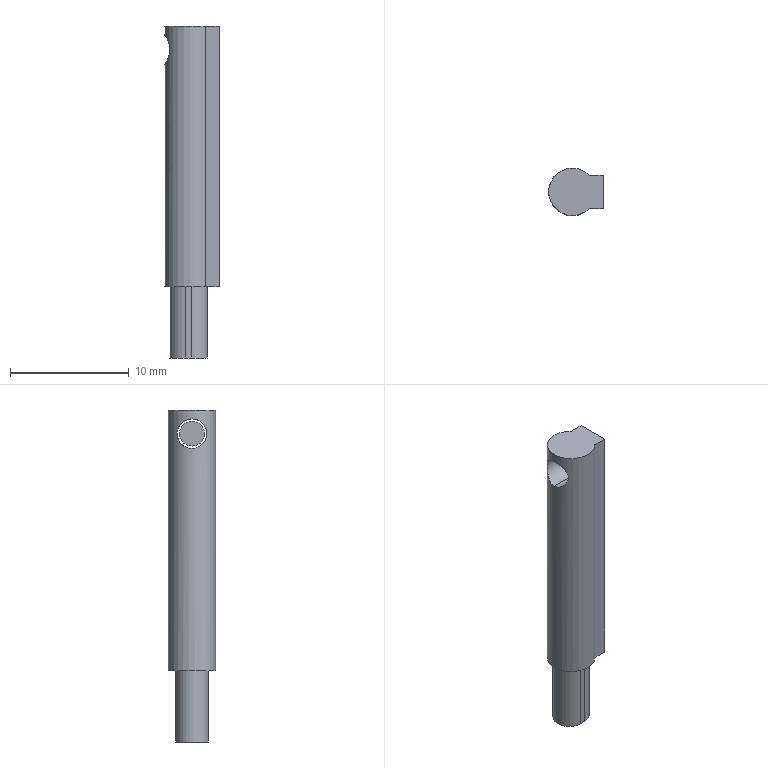Part | SolidWorks | features BaseBody 2 | 2 solids | 18 faces | box 4.6 x 4 x 28 mm | volume 348.237 mm3 | plane 10 | cylinder 8 | commonest cylinder face diameters 2.7 x3 2.1 x2 2.5 x2 4 x1
STEP:
#1=CARTESIAN_POINT('',(14.5,-5.5,-12.25));
#2=VERTEX_POINT('',#1);
#3=CARTESIAN_POINT('',(14.5,-5.5,-14.75));
#4=VERTEX_POINT('',#3);
#5=CARTESIAN_POINT('',(14.5,-5.5,-12.25));
#6=CARTESIAN_POINT('',(14.5,-5.585,-12.25));
#7=CARTESIAN_POINT('',(14.505,-5.668,-12.259));
#8=CARTESIAN_POINT('',(14.526,-5.832,-12.292));
#9=CARTESIAN_POINT('',(14.541,-5.912,-12.317));
#10=CARTESIAN_POINT('',(14.598,-6.138,-12.413));
#11=CARTESIAN_POINT('',(14.651,-6.274,-12.505));
#12=CARTESIAN_POINT('',(14.762,-6.498,-12.73));
#13=CARTESIAN_POINT('',(14.82,-6.588,-12.864));
#14=CARTESIAN_POINT('',(14.909,-6.714,-13.162));
#15=CARTESIAN_POINT('',(14.939,-6.75,-13.33));
#16=CARTESIAN_POINT('',(14.939,-6.75,-13.669));
#17=CARTESIAN_POINT('',(14.91,-6.715,-13.836));
#18=CARTESIAN_POINT('',(14.821,-6.589,-14.135));
#19=CARTESIAN_POINT('',(14.762,-6.498,-14.269));
#20=CARTESIAN_POINT('',(14.651,-6.272,-14.496));
#21=CARTESIAN_POINT('',(14.599,-6.14,-14.586));
#22=CARTESIAN_POINT('',(14.522,-5.835,-14.716));
#23=CARTESIAN_POINT('',(14.5,-5.671,-14.75));
#24=CARTESIAN_POINT('',(14.5,-5.5,-14.75));
#25=B_SPLINE_CURVE_WITH_KNOTS('',3,(#5,#6,#7,#8,#9,#10,#11,#12,#13,#14,#15,#16,#17,#18,#19,#20,#21,#22,#23,#24),.UNSPECIFIED.,.F.,.F.,(4,2,2,2,2,2,2,2,2,4),(0.,0.0002513,0.0005026,0.001005,0.001508,0.00201,0.002513,0.003016,0.003518,0.004021),.UNSPECIFIED.);
#26=EDGE_CURVE('',#2,#4,#25,.T.);
#27=ORIENTED_EDGE('',*,*,#26,.F.);
#28=CARTESIAN_POINT('',(19.1,-5.5,-12.25));
#29=VERTEX_POINT('',#28);
#30=CARTESIAN_POINT('',(19.1,-5.5,-12.25));
#31=DIRECTION('',(1.,0.,0.));
#32=VECTOR('',#31,1000.);
#33=LINE('',#30,#32);
#34=EDGE_CURVE('',#2,#29,#33,.T.);
#35=ORIENTED_EDGE('',*,*,#34,.T.);
#36=CARTESIAN_POINT('',(19.1,-5.5,-14.75));
#37=VERTEX_POINT('',#36);
#38=CARTESIAN_POINT('',(19.1,-5.5,-13.5));
#39=DIRECTION('',(-1.,0.,0.));
#40=DIRECTION('',(0.,0.,-1.));
#41=AXIS2_PLACEMENT_3D('',#38,#39,#40);
#42=CIRCLE('',#41,1.25);
#43=EDGE_CURVE('',#37,#29,#42,.T.);
#44=ORIENTED_EDGE('',*,*,#43,.F.);
#45=CARTESIAN_POINT('',(19.1,-5.5,-14.75));
#46=DIRECTION('',(1.,0.,0.));
#47=VECTOR('',#46,1000.);
#48=LINE('',#45,#47);
#49=EDGE_CURVE('',#4,#37,#48,.T.);
#50=ORIENTED_EDGE('',*,*,#49,.F.);
#51=EDGE_LOOP('',(#27,#35,#44,#50));
#52=FACE_OUTER_BOUND('',#51,.T.);
#53=CARTESIAN_POINT('',(19.1,-5.5,-13.5));
#54=DIRECTION('',(1.,0.,0.));
#55=DIRECTION('',(0.,0.,-1.));
#56=AXIS2_PLACEMENT_3D('',#53,#54,#55);
#57=CYLINDRICAL_SURFACE('',#56,1.25);
#58=ADVANCED_FACE('',(#52),#57,.F.);
#59=CARTESIAN_POINT('',(16.75,-6.85,-39.5));
#60=VERTEX_POINT('',#59);
#61=CARTESIAN_POINT('',(18.1,-5.5,-39.5));
#62=VERTEX_POINT('',#61);
#63=CARTESIAN_POINT('',(16.75,-5.5,-39.5));
#64=DIRECTION('',(0.,0.,1.));
#65=DIRECTION('',(1.,0.,0.));
#66=AXIS2_PLACEMENT_3D('',#63,#64,#65);
#67=CIRCLE('',#66,1.35);
#68=EDGE_CURVE('',#60,#62,#67,.T.);
#69=ORIENTED_EDGE('',*,*,#68,.T.);
#70=CARTESIAN_POINT('',(18.1,-5.5,-33.5));
#71=VERTEX_POINT('',#70);
#72=CARTESIAN_POINT('',(18.1,-5.5,-39.5));
#73=DIRECTION('',(0.,0.,1.));
#74=VECTOR('',#73,1000.);
#75=LINE('',#72,#74);
#76=EDGE_CURVE('',#62,#71,#75,.T.);
#77=ORIENTED_EDGE('',*,*,#76,.T.);
#78=CARTESIAN_POINT('',(16.75,-6.85,-33.5));
#79=VERTEX_POINT('',#78);
#80=CARTESIAN_POINT('',(16.75,-5.5,-33.5));
#81=DIRECTION('',(0.,0.,-1.));
#82=DIRECTION('',(1.,0.,0.));
#83=AXIS2_PLACEMENT_3D('',#80,#81,#82);
#84=CIRCLE('',#83,1.35);
#85=EDGE_CURVE('',#71,#79,#84,.T.);
#86=ORIENTED_EDGE('',*,*,#85,.T.);
#87=CARTESIAN_POINT('',(16.75,-6.85,-39.5));
#88=DIRECTION('',(0.,0.,-1.));
#89=VECTOR('',#88,1000.);
#90=LINE('',#87,#89);
#91=EDGE_CURVE('',#79,#60,#90,.T.);
#92=ORIENTED_EDGE('',*,*,#91,.T.);
#93=EDGE_LOOP('',(#69,#77,#86,#92));
#94=FACE_OUTER_BOUND('',#93,.T.);
#95=CARTESIAN_POINT('',(16.75,-5.5,-39.5));
#96=DIRECTION('',(0.,0.,1.));
#97=DIRECTION('',(1.,0.,0.));
#98=AXIS2_PLACEMENT_3D('',#95,#96,#97);
#99=CYLINDRICAL_SURFACE('',#98,1.35);
#100=ADVANCED_FACE('',(#94),#99,.T.);
#101=CARTESIAN_POINT('',(17.928,-4.1,-33.5));
#102=VERTEX_POINT('',#101);
#103=CARTESIAN_POINT('',(17.928,-6.9,-33.5));
#104=VERTEX_POINT('',#103);
#105=CARTESIAN_POINT('',(16.5,-5.5,-33.5));
#106=DIRECTION('',(0.,0.,1.));
#107=DIRECTION('',(1.,0.,0.));
#108=AXIS2_PLACEMENT_3D('',#105,#106,#107);
#109=CIRCLE('',#108,2.);
#110=EDGE_CURVE('',#102,#104,#109,.T.);
#111=ORIENTED_EDGE('',*,*,#110,.T.);
#112=CARTESIAN_POINT('',(17.928,-6.9,-11.5));
#113=VERTEX_POINT('',#112);
#114=CARTESIAN_POINT('',(17.928,-6.9,-33.5));
#115=DIRECTION('',(0.,0.,1.));
#116=VECTOR('',#115,1000.);
#117=LINE('',#114,#116);
#118=EDGE_CURVE('',#104,#113,#117,.T.);
#119=ORIENTED_EDGE('',*,*,#118,.T.);
#120=CARTESIAN_POINT('',(17.928,-4.1,-11.5));
#121=VERTEX_POINT('',#120);
#122=CARTESIAN_POINT('',(16.5,-5.5,-11.5));
#123=DIRECTION('',(0.,0.,-1.));
#124=DIRECTION('',(1.,0.,0.));
#125=AXIS2_PLACEMENT_3D('',#122,#123,#124);
#126=CIRCLE('',#125,2.);
#127=EDGE_CURVE('',#113,#121,#126,.T.);
#128=ORIENTED_EDGE('',*,*,#127,.T.);
#129=CARTESIAN_POINT('',(17.928,-4.1,-33.5));
#130=DIRECTION('',(0.,0.,-1.));
#131=VECTOR('',#130,1000.);
#132=LINE('',#129,#131);
#133=EDGE_CURVE('',#121,#102,#132,.T.);
#134=ORIENTED_EDGE('',*,*,#133,.T.);
#135=EDGE_LOOP('',(#111,#119,#128,#134));
#136=FACE_OUTER_BOUND('',#135,.T.);
#137=CARTESIAN_POINT('',(14.5,-5.5,-14.75));
#138=CARTESIAN_POINT('',(14.5,-5.415,-14.75));
#139=CARTESIAN_POINT('',(14.505,-5.332,-14.741));
#140=CARTESIAN_POINT('',(14.526,-5.168,-14.708));
#141=CARTESIAN_POINT('',(14.541,-5.088,-14.683));
#142=CARTESIAN_POINT('',(14.598,-4.862,-14.587));
#143=CARTESIAN_POINT('',(14.651,-4.726,-14.495));
#144=CARTESIAN_POINT('',(14.762,-4.502,-14.27));
#145=CARTESIAN_POINT('',(14.82,-4.412,-14.136));
#146=CARTESIAN_POINT('',(14.909,-4.286,-13.838));
#147=CARTESIAN_POINT('',(14.939,-4.25,-13.67));
#148=CARTESIAN_POINT('',(14.939,-4.25,-13.331));
#149=CARTESIAN_POINT('',(14.91,-4.285,-13.164));
#150=CARTESIAN_POINT('',(14.821,-4.411,-12.865));
#151=CARTESIAN_POINT('',(14.762,-4.502,-12.731));
#152=CARTESIAN_POINT('',(14.651,-4.728,-12.504));
#153=CARTESIAN_POINT('',(14.599,-4.86,-12.414));
#154=CARTESIAN_POINT('',(14.541,-5.089,-12.317));
#155=CARTESIAN_POINT('',(14.526,-5.168,-12.292));
#156=CARTESIAN_POINT('',(14.506,-5.33,-12.259));
#157=CARTESIAN_POINT('',(14.5,-5.415,-12.25));
#158=CARTESIAN_POINT('',(14.5,-5.5,-12.25));
#159=B_SPLINE_CURVE_WITH_KNOTS('',3,(#137,#138,#139,#140,#141,#142,#143,#144,#145,#146,#147,#148,#149,#150,#151,#152,#153,#154,#155,#156,#157,#158),.UNSPECIFIED.,.F.,.F.,(4,2,2,2,2,2,2,2,2,2,4),(0.004021,0.004271,0.004522,0.005024,0.005525,0.006027,0.006529,0.00703,0.007532,0.007783,0.008033),.UNSPECIFIED.);
#160=EDGE_CURVE('',#4,#2,#159,.T.);
#161=ORIENTED_EDGE('',*,*,#160,.T.);
#162=ORIENTED_EDGE('',*,*,#26,.T.);
#163=EDGE_LOOP('',(#161,#162));
#164=FACE_BOUND('',#163,.T.);
#165=CARTESIAN_POINT('',(16.5,-5.5,-33.5));
#166=DIRECTION('',(0.,0.,1.));
#167=DIRECTION('',(1.,0.,0.));
#168=AXIS2_PLACEMENT_3D('',#165,#166,#167);
#169=CYLINDRICAL_SURFACE('',#168,2.);
#170=ADVANCED_FACE('',(#136,#164),#169,.T.);
#171=CARTESIAN_POINT('',(19.1,-6.9,-33.5));
#172=VERTEX_POINT('',#171);
#173=CARTESIAN_POINT('',(17.928,-6.9,-33.5));
#174=DIRECTION('',(1.,0.,0.));
#175=VECTOR('',#174,1000.);
#176=LINE('',#173,#175);
#177=EDGE_CURVE('',#104,#172,#176,.T.);
#178=ORIENTED_EDGE('',*,*,#177,.T.);
#179=CARTESIAN_POINT('',(19.1,-6.9,-11.5));
#180=VERTEX_POINT('',#179);
#181=CARTESIAN_POINT('',(19.1,-6.9,-33.5));
#182=DIRECTION('',(0.,0.,1.));
#183=VECTOR('',#182,1000.);
#184=LINE('',#181,#183);
#185=EDGE_CURVE('',#172,#180,#184,.T.);
#186=ORIENTED_EDGE('',*,*,#185,.T.);
#187=CARTESIAN_POINT('',(17.928,-6.9,-11.5));
#188=DIRECTION('',(-1.,0.,0.));
#189=VECTOR('',#188,1000.);
#190=LINE('',#187,#189);
#191=EDGE_CURVE('',#180,#113,#190,.T.);
#192=ORIENTED_EDGE('',*,*,#191,.T.);
#193=ORIENTED_EDGE('',*,*,#118,.F.);
#194=EDGE_LOOP('',(#178,#186,#192,#193));
#195=FACE_OUTER_BOUND('',#194,.T.);
#196=CARTESIAN_POINT('',(17.928,-6.9,-33.5));
#197=DIRECTION('',(0.,-1.,0.));
#198=DIRECTION('',(1.,0.,0.));
#199=AXIS2_PLACEMENT_3D('',#196,#197,#198);
#200=PLANE('',#199);
#201=ADVANCED_FACE('',(#195),#200,.T.);
#202=CARTESIAN_POINT('',(16.25,-6.85,-33.5));
#203=VERTEX_POINT('',#202);
#204=CARTESIAN_POINT('',(16.25,-6.85,-33.5));
#205=DIRECTION('',(1.,0.,0.));
#206=VECTOR('',#205,1000.);
#207=LINE('',#204,#206);
#208=EDGE_CURVE('',#203,#79,#207,.T.);
#209=ORIENTED_EDGE('',*,*,#208,.T.);
#210=ORIENTED_EDGE('',*,*,#85,.F.);
#211=CARTESIAN_POINT('',(16.75,-4.15,-33.5));
#212=VERTEX_POINT('',#211);
#213=CARTESIAN_POINT('',(16.75,-5.5,-33.5));
#214=DIRECTION('',(0.,0.,-1.));
#215=DIRECTION('',(1.,0.,0.));
#216=AXIS2_PLACEMENT_3D('',#213,#214,#215);
#217=CIRCLE('',#216,1.35);
#218=EDGE_CURVE('',#212,#71,#217,.T.);
#219=ORIENTED_EDGE('',*,*,#218,.F.);
#220=CARTESIAN_POINT('',(16.25,-4.15,-33.5));
#221=VERTEX_POINT('',#220);
#222=CARTESIAN_POINT('',(16.75,-4.15,-33.5));
#223=DIRECTION('',(-1.,0.,0.));
#224=VECTOR('',#223,1000.);
#225=LINE('',#222,#224);
#226=EDGE_CURVE('',#212,#221,#225,.T.);
#227=ORIENTED_EDGE('',*,*,#226,.T.);
#228=CARTESIAN_POINT('',(16.25,-5.5,-33.5));
#229=DIRECTION('',(0.,0.,-1.));
#230=DIRECTION('',(1.,0.,0.));
#231=AXIS2_PLACEMENT_3D('',#228,#229,#230);
#232=CIRCLE('',#231,1.35);
#233=EDGE_CURVE('',#203,#221,#232,.T.);
#234=ORIENTED_EDGE('',*,*,#233,.F.);
#235=EDGE_LOOP('',(#209,#210,#219,#227,#234));
#236=FACE_BOUND('',#235,.T.);
#237=ORIENTED_EDGE('',*,*,#110,.F.);
#238=CARTESIAN_POINT('',(19.1,-4.1,-33.5));
#239=VERTEX_POINT('',#238);
#240=CARTESIAN_POINT('',(16.5,-4.1,-33.5));
#241=DIRECTION('',(-1.,0.,0.));
#242=VECTOR('',#241,1000.);
#243=LINE('',#240,#242);
#244=EDGE_CURVE('',#239,#102,#243,.T.);
#245=ORIENTED_EDGE('',*,*,#244,.F.);
#246=CARTESIAN_POINT('',(19.1,-5.5,-33.5));
#247=DIRECTION('',(0.,1.,0.));
#248=VECTOR('',#247,1000.);
#249=LINE('',#246,#248);
#250=EDGE_CURVE('',#172,#239,#249,.T.);
#251=ORIENTED_EDGE('',*,*,#250,.F.);
#252=ORIENTED_EDGE('',*,*,#177,.F.);
#253=EDGE_LOOP('',(#237,#245,#251,#252));
#254=FACE_OUTER_BOUND('',#253,.T.);
#255=CARTESIAN_POINT('',(16.5,-5.5,-33.5));
#256=DIRECTION('',(0.,0.,1.));
#257=DIRECTION('',(1.,0.,0.));
#258=AXIS2_PLACEMENT_3D('',#255,#256,#257);
#259=PLANE('',#258);
#260=ADVANCED_FACE('',(#236,#254),#259,.F.);
#261=ORIENTED_EDGE('',*,*,#244,.T.);
#262=ORIENTED_EDGE('',*,*,#133,.F.);
#263=CARTESIAN_POINT('',(19.1,-4.1,-11.5));
#264=VERTEX_POINT('',#263);
#265=CARTESIAN_POINT('',(19.1,-4.1,-11.5));
#266=DIRECTION('',(1.,0.,0.));
#267=VECTOR('',#266,1000.);
#268=LINE('',#265,#267);
#269=EDGE_CURVE('',#121,#264,#268,.T.);
#270=ORIENTED_EDGE('',*,*,#269,.T.);
#271=CARTESIAN_POINT('',(19.1,-4.1,-33.5));
#272=DIRECTION('',(0.,0.,-1.));
#273=VECTOR('',#272,1000.);
#274=LINE('',#271,#273);
#275=EDGE_CURVE('',#264,#239,#274,.T.);
#276=ORIENTED_EDGE('',*,*,#275,.T.);
#277=EDGE_LOOP('',(#261,#262,#270,#276));
#278=FACE_OUTER_BOUND('',#277,.T.);
#279=CARTESIAN_POINT('',(19.1,-4.1,-33.5));
#280=DIRECTION('',(0.,1.,0.));
#281=DIRECTION('',(-1.,0.,0.));
#282=AXIS2_PLACEMENT_3D('',#279,#280,#281);
#283=PLANE('',#282);
#284=ADVANCED_FACE('',(#278),#283,.T.);
#285=ORIENTED_EDGE('',*,*,#269,.F.);
#286=ORIENTED_EDGE('',*,*,#127,.F.);
#287=ORIENTED_EDGE('',*,*,#191,.F.);
#288=CARTESIAN_POINT('',(19.1,-5.5,-11.5));
#289=DIRECTION('',(0.,1.,0.));
#290=VECTOR('',#289,1000.);
#291=LINE('',#288,#290);
#292=EDGE_CURVE('',#180,#264,#291,.T.);
#293=ORIENTED_EDGE('',*,*,#292,.T.);
#294=EDGE_LOOP('',(#285,#286,#287,#293));
#295=FACE_OUTER_BOUND('',#294,.T.);
#296=CARTESIAN_POINT('',(16.5,-5.5,-11.5));
#297=DIRECTION('',(0.,0.,1.));
#298=DIRECTION('',(1.,0.,0.));
#299=AXIS2_PLACEMENT_3D('',#296,#297,#298);
#300=PLANE('',#299);
#301=ADVANCED_FACE('',(#295),#300,.T.);
#302=ORIENTED_EDGE('',*,*,#34,.F.);
#303=ORIENTED_EDGE('',*,*,#160,.F.);
#304=ORIENTED_EDGE('',*,*,#49,.T.);
#305=CARTESIAN_POINT('',(19.1,-5.5,-13.5));
#306=DIRECTION('',(-1.,0.,0.));
#307=DIRECTION('',(0.,0.,-1.));
#308=AXIS2_PLACEMENT_3D('',#305,#306,#307);
#309=CIRCLE('',#308,1.25);
#310=EDGE_CURVE('',#29,#37,#309,.T.);
#311=ORIENTED_EDGE('',*,*,#310,.F.);
#312=EDGE_LOOP('',(#302,#303,#304,#311));
#313=FACE_OUTER_BOUND('',#312,.T.);
#314=CARTESIAN_POINT('',(19.1,-5.5,-13.5));
#315=DIRECTION('',(1.,0.,0.));
#316=DIRECTION('',(0.,0.,-1.));
#317=AXIS2_PLACEMENT_3D('',#314,#315,#316);
#318=CYLINDRICAL_SURFACE('',#317,1.25);
#319=ADVANCED_FACE('',(#313),#318,.F.);
#320=ORIENTED_EDGE('',*,*,#250,.T.);
#321=ORIENTED_EDGE('',*,*,#275,.F.);
#322=ORIENTED_EDGE('',*,*,#292,.F.);
#323=ORIENTED_EDGE('',*,*,#185,.F.);
#324=EDGE_LOOP('',(#320,#321,#322,#323));
#325=FACE_OUTER_BOUND('',#324,.T.);
#326=ORIENTED_EDGE('',*,*,#43,.T.);
#327=ORIENTED_EDGE('',*,*,#310,.T.);
#328=EDGE_LOOP('',(#326,#327));
#329=FACE_BOUND('',#328,.T.);
#330=CARTESIAN_POINT('',(19.1,-6.9,-33.5));
#331=DIRECTION('',(1.,0.,0.));
#332=DIRECTION('',(0.,0.,-1.));
#333=AXIS2_PLACEMENT_3D('',#330,#331,#332);
#334=PLANE('',#333);
#335=ADVANCED_FACE('',(#325,#329),#334,.T.);
#336=CARTESIAN_POINT('',(16.25,-4.15,-39.5));
#337=VERTEX_POINT('',#336);
#338=CARTESIAN_POINT('',(16.25,-6.85,-39.5));
#339=VERTEX_POINT('',#338);
#340=CARTESIAN_POINT('',(16.25,-5.5,-39.5));
#341=DIRECTION('',(0.,0.,1.));
#342=DIRECTION('',(1.,0.,0.));
#343=AXIS2_PLACEMENT_3D('',#340,#341,#342);
#344=CIRCLE('',#343,1.35);
#345=EDGE_CURVE('',#337,#339,#344,.T.);
#346=ORIENTED_EDGE('',*,*,#345,.T.);
#347=CARTESIAN_POINT('',(16.25,-6.85,-39.5));
#348=DIRECTION('',(0.,0.,1.));
#349=VECTOR('',#348,1000.);
#350=LINE('',#347,#349);
#351=EDGE_CURVE('',#339,#203,#350,.T.);
#352=ORIENTED_EDGE('',*,*,#351,.T.);
#353=ORIENTED_EDGE('',*,*,#233,.T.);
#354=CARTESIAN_POINT('',(16.25,-4.15,-39.5));
#355=DIRECTION('',(0.,0.,-1.));
#356=VECTOR('',#355,1000.);
#357=LINE('',#354,#356);
#358=EDGE_CURVE('',#221,#337,#357,.T.);
#359=ORIENTED_EDGE('',*,*,#358,.T.);
#360=EDGE_LOOP('',(#346,#352,#353,#359));
#361=FACE_OUTER_BOUND('',#360,.T.);
#362=CARTESIAN_POINT('',(16.25,-5.5,-39.5));
#363=DIRECTION('',(0.,0.,1.));
#364=DIRECTION('',(1.,0.,0.));
#365=AXIS2_PLACEMENT_3D('',#362,#363,#364);
#366=CYLINDRICAL_SURFACE('',#365,1.35);
#367=ADVANCED_FACE('',(#361),#366,.T.);
#368=ORIENTED_EDGE('',*,*,#76,.F.);
#369=CARTESIAN_POINT('',(16.75,-4.15,-39.5));
#370=VERTEX_POINT('',#369);
#371=CARTESIAN_POINT('',(16.75,-5.5,-39.5));
#372=DIRECTION('',(0.,0.,1.));
#373=DIRECTION('',(1.,0.,0.));
#374=AXIS2_PLACEMENT_3D('',#371,#372,#373);
#375=CIRCLE('',#374,1.35);
#376=EDGE_CURVE('',#62,#370,#375,.T.);
#377=ORIENTED_EDGE('',*,*,#376,.T.);
#378=CARTESIAN_POINT('',(16.75,-4.15,-39.5));
#379=DIRECTION('',(0.,0.,1.));
#380=VECTOR('',#379,1000.);
#381=LINE('',#378,#380);
#382=EDGE_CURVE('',#370,#212,#381,.T.);
#383=ORIENTED_EDGE('',*,*,#382,.T.);
#384=ORIENTED_EDGE('',*,*,#218,.T.);
#385=EDGE_LOOP('',(#368,#377,#383,#384));
#386=FACE_OUTER_BOUND('',#385,.T.);
#387=CARTESIAN_POINT('',(16.75,-5.5,-39.5));
#388=DIRECTION('',(0.,0.,1.));
#389=DIRECTION('',(1.,0.,0.));
#390=AXIS2_PLACEMENT_3D('',#387,#388,#389);
#391=CYLINDRICAL_SURFACE('',#390,1.35);
#392=ADVANCED_FACE('',(#386),#391,.T.);
#393=ORIENTED_EDGE('',*,*,#351,.F.);
#394=CARTESIAN_POINT('',(16.25,-6.85,-39.5));
#395=DIRECTION('',(-1.,0.,0.));
#396=VECTOR('',#395,1000.);
#397=LINE('',#394,#396);
#398=EDGE_CURVE('',#60,#339,#397,.T.);
#399=ORIENTED_EDGE('',*,*,#398,.F.);
#400=ORIENTED_EDGE('',*,*,#91,.F.);
#401=ORIENTED_EDGE('',*,*,#208,.F.);
#402=EDGE_LOOP('',(#393,#399,#400,#401));
#403=FACE_OUTER_BOUND('',#402,.T.);
#404=CARTESIAN_POINT('',(16.25,-6.85,-39.5));
#405=DIRECTION('',(0.,1.,0.));
#406=DIRECTION('',(0.,0.,1.));
#407=AXIS2_PLACEMENT_3D('',#404,#405,#406);
#408=PLANE('',#407);
#409=ADVANCED_FACE('',(#403),#408,.F.);
#410=CARTESIAN_POINT('',(16.25,-4.15,-39.5));
#411=DIRECTION('',(-1.,0.,0.));
#412=VECTOR('',#411,1000.);
#413=LINE('',#410,#412);
#414=EDGE_CURVE('',#370,#337,#413,.T.);
#415=ORIENTED_EDGE('',*,*,#414,.F.);
#416=ORIENTED_EDGE('',*,*,#376,.F.);
#417=ORIENTED_EDGE('',*,*,#68,.F.);
#418=ORIENTED_EDGE('',*,*,#398,.T.);
#419=ORIENTED_EDGE('',*,*,#345,.F.);
#420=EDGE_LOOP('',(#415,#416,#417,#418,#419));
#421=FACE_OUTER_BOUND('',#420,.T.);
#422=CARTESIAN_POINT('',(16.25,-5.5,-39.5));
#423=DIRECTION('',(0.,0.,1.));
#424=DIRECTION('',(1.,0.,0.));
#425=AXIS2_PLACEMENT_3D('',#422,#423,#424);
#426=PLANE('',#425);
#427=ADVANCED_FACE('',(#421),#426,.F.);
#428=ORIENTED_EDGE('',*,*,#382,.F.);
#429=ORIENTED_EDGE('',*,*,#414,.T.);
#430=ORIENTED_EDGE('',*,*,#358,.F.);
#431=ORIENTED_EDGE('',*,*,#226,.F.);
#432=EDGE_LOOP('',(#428,#429,#430,#431));
#433=FACE_OUTER_BOUND('',#432,.T.);
#434=CARTESIAN_POINT('',(16.75,-4.15,-39.5));
#435=DIRECTION('',(0.,-1.,0.));
#436=DIRECTION('',(0.,0.,-1.));
#437=AXIS2_PLACEMENT_3D('',#434,#435,#436);
#438=PLANE('',#437);
#439=ADVANCED_FACE('',(#433),#438,.F.);
#440=CLOSED_SHELL('',(#58,#100,#170,#201,#260,#284,#301,#319,#335,#367,#392,#409,#427,#439));
#441=MANIFOLD_SOLID_BREP('',#440);
#442=CARTESIAN_POINT('',(18.1,-5.5,-12.45));
#443=VERTEX_POINT('',#442);
#444=CARTESIAN_POINT('',(18.1,-5.5,-14.55));
#445=VERTEX_POINT('',#444);
#446=CARTESIAN_POINT('',(18.1,-5.5,-13.5));
#447=DIRECTION('',(-1.,0.,0.));
#448=DIRECTION('',(0.,0.,-1.));
#449=AXIS2_PLACEMENT_3D('',#446,#447,#448);
#450=CIRCLE('',#449,1.05);
#451=EDGE_CURVE('',#443,#445,#450,.T.);
#452=ORIENTED_EDGE('',*,*,#451,.F.);
#453=CARTESIAN_POINT('',(19.1,-5.5,-12.45));
#454=VERTEX_POINT('',#453);
#455=CARTESIAN_POINT('',(18.1,-5.5,-12.45));
#456=DIRECTION('',(1.,0.,0.));
#457=VECTOR('',#456,1000.);
#458=LINE('',#455,#457);
#459=EDGE_CURVE('',#443,#454,#458,.T.);
#460=ORIENTED_EDGE('',*,*,#459,.T.);
#461=CARTESIAN_POINT('',(19.1,-5.5,-14.55));
#462=VERTEX_POINT('',#461);
#463=CARTESIAN_POINT('',(19.1,-5.5,-13.5));
#464=DIRECTION('',(-1.,0.,0.));
#465=DIRECTION('',(0.,0.,-1.));
#466=AXIS2_PLACEMENT_3D('',#463,#464,#465);
#467=CIRCLE('',#466,1.05);
#468=EDGE_CURVE('',#454,#462,#467,.T.);
#469=ORIENTED_EDGE('',*,*,#468,.T.);
#470=CARTESIAN_POINT('',(18.1,-5.5,-14.55));
#471=DIRECTION('',(1.,0.,0.));
#472=VECTOR('',#471,1000.);
#473=LINE('',#470,#472);
#474=EDGE_CURVE('',#445,#462,#473,.T.);
#475=ORIENTED_EDGE('',*,*,#474,.F.);
#476=EDGE_LOOP('',(#452,#460,#469,#475));
#477=FACE_OUTER_BOUND('',#476,.T.);
#478=CARTESIAN_POINT('',(18.1,-5.5,-13.5));
#479=DIRECTION('',(1.,0.,0.));
#480=DIRECTION('',(0.,0.,-1.));
#481=AXIS2_PLACEMENT_3D('',#478,#479,#480);
#482=CYLINDRICAL_SURFACE('',#481,1.05);
#483=ADVANCED_FACE('',(#477),#482,.T.);
#484=CARTESIAN_POINT('',(18.1,-5.5,-13.5));
#485=DIRECTION('',(-1.,0.,0.));
#486=DIRECTION('',(0.,0.,-1.));
#487=AXIS2_PLACEMENT_3D('',#484,#485,#486);
#488=CIRCLE('',#487,1.05);
#489=EDGE_CURVE('',#445,#443,#488,.T.);
#490=ORIENTED_EDGE('',*,*,#489,.T.);
#491=ORIENTED_EDGE('',*,*,#451,.T.);
#492=EDGE_LOOP('',(#490,#491));
#493=FACE_OUTER_BOUND('',#492,.T.);
#494=CARTESIAN_POINT('',(18.1,-4.45,-13.5));
#495=DIRECTION('',(-1.,0.,0.));
#496=DIRECTION('',(0.,0.,1.));
#497=AXIS2_PLACEMENT_3D('',#494,#495,#496);
#498=PLANE('',#497);
#499=ADVANCED_FACE('',(#493),#498,.T.);
#500=ORIENTED_EDGE('',*,*,#459,.F.);
#501=ORIENTED_EDGE('',*,*,#489,.F.);
#502=ORIENTED_EDGE('',*,*,#474,.T.);
#503=CARTESIAN_POINT('',(19.1,-5.5,-13.5));
#504=DIRECTION('',(-1.,0.,0.));
#505=DIRECTION('',(0.,0.,-1.));
#506=AXIS2_PLACEMENT_3D('',#503,#504,#505);
#507=CIRCLE('',#506,1.05);
#508=EDGE_CURVE('',#462,#454,#507,.T.);
#509=ORIENTED_EDGE('',*,*,#508,.T.);
#510=EDGE_LOOP('',(#500,#501,#502,#509));
#511=FACE_OUTER_BOUND('',#510,.T.);
#512=CARTESIAN_POINT('',(18.1,-5.5,-13.5));
#513=DIRECTION('',(1.,0.,0.));
#514=DIRECTION('',(0.,0.,-1.));
#515=AXIS2_PLACEMENT_3D('',#512,#513,#514);
#516=CYLINDRICAL_SURFACE('',#515,1.05);
#517=ADVANCED_FACE('',(#511),#516,.T.);
#518=ORIENTED_EDGE('',*,*,#508,.F.);
#519=ORIENTED_EDGE('',*,*,#468,.F.);
#520=EDGE_LOOP('',(#518,#519));
#521=FACE_OUTER_BOUND('',#520,.T.);
#522=CARTESIAN_POINT('',(19.1,-5.5,-13.5));
#523=DIRECTION('',(1.,0.,0.));
#524=DIRECTION('',(0.,0.,-1.));
#525=AXIS2_PLACEMENT_3D('',#522,#523,#524);
#526=PLANE('',#525);
#527=ADVANCED_FACE('',(#521),#526,.T.);
#528=CLOSED_SHELL('',(#483,#499,#517,#527));
#529=MANIFOLD_SOLID_BREP('',#528);
#530=CARTESIAN_POINT('',(0.,0.,0.));
#531=DIRECTION('',(0.,0.,1.));
#532=DIRECTION('',(1.,0.,0.));
#533=AXIS2_PLACEMENT_3D('',#530,#531,#532);
#534=(LENGTH_UNIT()NAMED_UNIT(*)SI_UNIT(.MILLI.,.METRE.));
#535=UNCERTAINTY_MEASURE_WITH_UNIT(LENGTH_MEASURE(0.00001),#534,'','');
#536=(NAMED_UNIT(*)PLANE_ANGLE_UNIT()SI_UNIT($,.RADIAN.));
#537=(NAMED_UNIT(*)SI_UNIT($,.STERADIAN.)SOLID_ANGLE_UNIT());
#538=(GEOMETRIC_REPRESENTATION_CONTEXT(3)GLOBAL_UNCERTAINTY_ASSIGNED_CONTEXT((#535))GLOBAL_UNIT_ASSIGNED_CONTEXT((#534,#536,#537))REPRESENTATION_CONTEXT('',''));
#539=ADVANCED_BREP_SHAPE_REPRESENTATION('',(#441,#529,#533),#538);